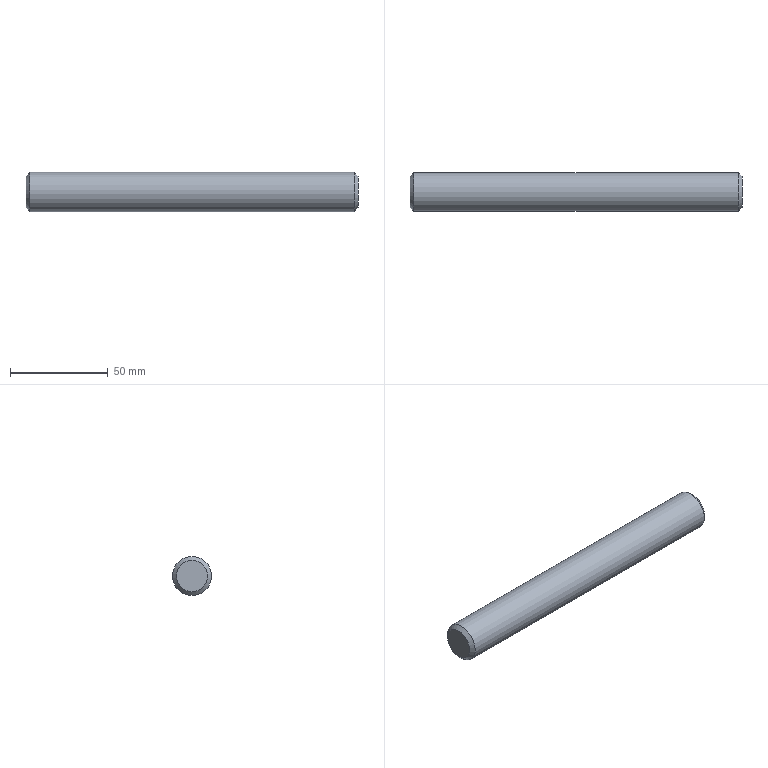Part | STEP file | solid 76 | 1 solid | 5 faces | box 170 x 20 x 20 mm | volume 53173 mm3 | plane 2 | cone 2 | cylinder 1 | commonest cylinder face diameters 20 x1